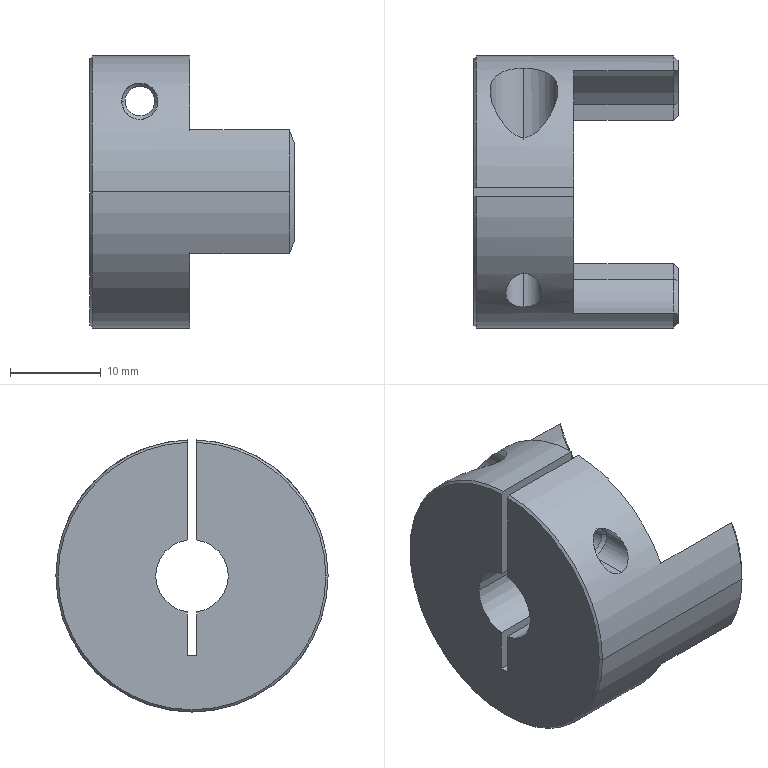Part | NX | 1 solid | 55 faces | box 22.5 x 30 x 29.992 mm | volume 7635 mm3 | cylinder 20 | plane 18 | cone 17 | commonest cylinder face diameters 4 x4 16.982 x4 8 x3 30 x3 3.242 x2 7.5 x2